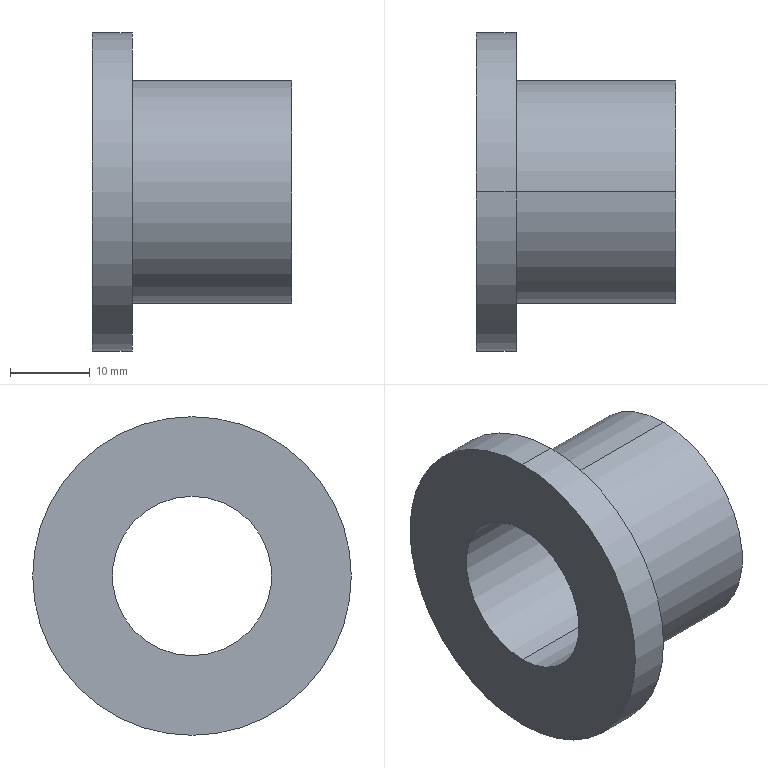Part | SolidWorks | features Revolution 1 | 1 solid | 9 faces | box 25 x 40 x 40 mm | volume 10744 mm3 | cylinder 6 | plane 3 | commonest cylinder face diameters 20 x2 28 x2 40 x2
STEP:
#1=CARTESIAN_POINT('',(25.,0.,24.));
#2=VERTEX_POINT('',#1);
#3=CARTESIAN_POINT('',(25.,0.,-4.));
#4=VERTEX_POINT('',#3);
#5=CARTESIAN_POINT('',(25.,0.,10.));
#6=DIRECTION('',(-1.,0.,0.));
#7=DIRECTION('',(0.,0.,1.));
#8=AXIS2_PLACEMENT_3D('',#5,#6,#7);
#9=CIRCLE('',#8,14.);
#10=EDGE_CURVE('',#2,#4,#9,.T.);
#11=ORIENTED_EDGE('',*,*,#10,.T.);
#12=CARTESIAN_POINT('',(5.,0.,-4.));
#13=VERTEX_POINT('',#12);
#14=CARTESIAN_POINT('',(0.,0.,-4.));
#15=DIRECTION('',(-1.,0.,0.));
#16=VECTOR('',#15,1000.);
#17=LINE('',#14,#16);
#18=EDGE_CURVE('',#4,#13,#17,.T.);
#19=ORIENTED_EDGE('',*,*,#18,.T.);
#20=CARTESIAN_POINT('',(5.,0.,24.));
#21=VERTEX_POINT('',#20);
#22=CARTESIAN_POINT('',(5.,0.,10.));
#23=DIRECTION('',(-1.,0.,0.));
#24=DIRECTION('',(0.,0.,1.));
#25=AXIS2_PLACEMENT_3D('',#22,#23,#24);
#26=CIRCLE('',#25,14.);
#27=EDGE_CURVE('',#21,#13,#26,.T.);
#28=ORIENTED_EDGE('',*,*,#27,.F.);
#29=CARTESIAN_POINT('',(0.,0.,24.));
#30=DIRECTION('',(-1.,0.,0.));
#31=VECTOR('',#30,1000.);
#32=LINE('',#29,#31);
#33=EDGE_CURVE('',#2,#21,#32,.T.);
#34=ORIENTED_EDGE('',*,*,#33,.F.);
#35=EDGE_LOOP('',(#11,#19,#28,#34));
#36=FACE_OUTER_BOUND('',#35,.T.);
#37=CARTESIAN_POINT('',(0.,0.,10.));
#38=DIRECTION('',(-1.,0.,0.));
#39=DIRECTION('',(0.,0.,1.));
#40=AXIS2_PLACEMENT_3D('',#37,#38,#39);
#41=CYLINDRICAL_SURFACE('',#40,14.);
#42=ADVANCED_FACE('',(#36),#41,.T.);
#43=CARTESIAN_POINT('',(5.,0.,30.));
#44=VERTEX_POINT('',#43);
#45=CARTESIAN_POINT('',(5.,0.,-10.));
#46=VERTEX_POINT('',#45);
#47=CARTESIAN_POINT('',(5.,0.,10.));
#48=DIRECTION('',(-1.,0.,0.));
#49=DIRECTION('',(0.,0.,1.));
#50=AXIS2_PLACEMENT_3D('',#47,#48,#49);
#51=CIRCLE('',#50,20.);
#52=EDGE_CURVE('',#44,#46,#51,.T.);
#53=ORIENTED_EDGE('',*,*,#52,.T.);
#54=CARTESIAN_POINT('',(0.,0.,-10.));
#55=VERTEX_POINT('',#54);
#56=CARTESIAN_POINT('',(0.,0.,-10.));
#57=DIRECTION('',(-1.,0.,0.));
#58=VECTOR('',#57,1000.);
#59=LINE('',#56,#58);
#60=EDGE_CURVE('',#46,#55,#59,.T.);
#61=ORIENTED_EDGE('',*,*,#60,.T.);
#62=CARTESIAN_POINT('',(0.,0.,30.));
#63=VERTEX_POINT('',#62);
#64=CARTESIAN_POINT('',(0.,0.,10.));
#65=DIRECTION('',(-1.,0.,0.));
#66=DIRECTION('',(0.,0.,1.));
#67=AXIS2_PLACEMENT_3D('',#64,#65,#66);
#68=CIRCLE('',#67,20.);
#69=EDGE_CURVE('',#63,#55,#68,.T.);
#70=ORIENTED_EDGE('',*,*,#69,.F.);
#71=CARTESIAN_POINT('',(0.,0.,30.));
#72=DIRECTION('',(-1.,0.,0.));
#73=VECTOR('',#72,1000.);
#74=LINE('',#71,#73);
#75=EDGE_CURVE('',#44,#63,#74,.T.);
#76=ORIENTED_EDGE('',*,*,#75,.F.);
#77=EDGE_LOOP('',(#53,#61,#70,#76));
#78=FACE_OUTER_BOUND('',#77,.T.);
#79=CARTESIAN_POINT('',(0.,0.,10.));
#80=DIRECTION('',(-1.,0.,0.));
#81=DIRECTION('',(0.,0.,1.));
#82=AXIS2_PLACEMENT_3D('',#79,#80,#81);
#83=CYLINDRICAL_SURFACE('',#82,20.);
#84=ADVANCED_FACE('',(#78),#83,.T.);
#85=CARTESIAN_POINT('',(25.,0.,0.));
#86=VERTEX_POINT('',#85);
#87=CARTESIAN_POINT('',(25.,0.,20.));
#88=VERTEX_POINT('',#87);
#89=CARTESIAN_POINT('',(25.,0.,10.));
#90=DIRECTION('',(-1.,0.,0.));
#91=DIRECTION('',(0.,0.,1.));
#92=AXIS2_PLACEMENT_3D('',#89,#90,#91);
#93=CIRCLE('',#92,10.);
#94=EDGE_CURVE('',#86,#88,#93,.T.);
#95=ORIENTED_EDGE('',*,*,#94,.F.);
#96=CARTESIAN_POINT('',(0.,0.,0.));
#97=VERTEX_POINT('',#96);
#98=CARTESIAN_POINT('',(0.,0.,0.));
#99=DIRECTION('',(-1.,0.,0.));
#100=VECTOR('',#99,1000.);
#101=LINE('',#98,#100);
#102=EDGE_CURVE('',#86,#97,#101,.T.);
#103=ORIENTED_EDGE('',*,*,#102,.T.);
#104=CARTESIAN_POINT('',(0.,0.,20.));
#105=VERTEX_POINT('',#104);
#106=CARTESIAN_POINT('',(0.,0.,10.));
#107=DIRECTION('',(-1.,0.,0.));
#108=DIRECTION('',(0.,0.,1.));
#109=AXIS2_PLACEMENT_3D('',#106,#107,#108);
#110=CIRCLE('',#109,10.);
#111=EDGE_CURVE('',#97,#105,#110,.T.);
#112=ORIENTED_EDGE('',*,*,#111,.T.);
#113=CARTESIAN_POINT('',(0.,0.,20.));
#114=DIRECTION('',(-1.,0.,0.));
#115=VECTOR('',#114,1000.);
#116=LINE('',#113,#115);
#117=EDGE_CURVE('',#88,#105,#116,.T.);
#118=ORIENTED_EDGE('',*,*,#117,.F.);
#119=EDGE_LOOP('',(#95,#103,#112,#118));
#120=FACE_OUTER_BOUND('',#119,.T.);
#121=CARTESIAN_POINT('',(0.,0.,10.));
#122=DIRECTION('',(-1.,0.,0.));
#123=DIRECTION('',(0.,0.,1.));
#124=AXIS2_PLACEMENT_3D('',#121,#122,#123);
#125=CYLINDRICAL_SURFACE('',#124,10.);
#126=ADVANCED_FACE('',(#120),#125,.F.);
#127=ORIENTED_EDGE('',*,*,#102,.F.);
#128=CARTESIAN_POINT('',(25.,0.,10.));
#129=DIRECTION('',(-1.,0.,0.));
#130=DIRECTION('',(0.,0.,1.));
#131=AXIS2_PLACEMENT_3D('',#128,#129,#130);
#132=CIRCLE('',#131,10.);
#133=EDGE_CURVE('',#88,#86,#132,.T.);
#134=ORIENTED_EDGE('',*,*,#133,.F.);
#135=ORIENTED_EDGE('',*,*,#117,.T.);
#136=CARTESIAN_POINT('',(0.,0.,10.));
#137=DIRECTION('',(-1.,0.,0.));
#138=DIRECTION('',(0.,0.,1.));
#139=AXIS2_PLACEMENT_3D('',#136,#137,#138);
#140=CIRCLE('',#139,10.);
#141=EDGE_CURVE('',#105,#97,#140,.T.);
#142=ORIENTED_EDGE('',*,*,#141,.T.);
#143=EDGE_LOOP('',(#127,#134,#135,#142));
#144=FACE_OUTER_BOUND('',#143,.T.);
#145=CARTESIAN_POINT('',(0.,0.,10.));
#146=DIRECTION('',(-1.,0.,0.));
#147=DIRECTION('',(0.,0.,1.));
#148=AXIS2_PLACEMENT_3D('',#145,#146,#147);
#149=CYLINDRICAL_SURFACE('',#148,10.);
#150=ADVANCED_FACE('',(#144),#149,.F.);
#151=ORIENTED_EDGE('',*,*,#141,.F.);
#152=ORIENTED_EDGE('',*,*,#111,.F.);
#153=EDGE_LOOP('',(#151,#152));
#154=FACE_BOUND('',#153,.T.);
#155=ORIENTED_EDGE('',*,*,#69,.T.);
#156=CARTESIAN_POINT('',(0.,0.,10.));
#157=DIRECTION('',(-1.,0.,0.));
#158=DIRECTION('',(0.,0.,1.));
#159=AXIS2_PLACEMENT_3D('',#156,#157,#158);
#160=CIRCLE('',#159,20.);
#161=EDGE_CURVE('',#55,#63,#160,.T.);
#162=ORIENTED_EDGE('',*,*,#161,.T.);
#163=EDGE_LOOP('',(#155,#162));
#164=FACE_OUTER_BOUND('',#163,.T.);
#165=CARTESIAN_POINT('',(0.,0.,0.));
#166=DIRECTION('',(1.,0.,0.));
#167=DIRECTION('',(0.,0.,-1.));
#168=AXIS2_PLACEMENT_3D('',#165,#166,#167);
#169=PLANE('',#168);
#170=ADVANCED_FACE('',(#154,#164),#169,.F.);
#171=ORIENTED_EDGE('',*,*,#60,.F.);
#172=CARTESIAN_POINT('',(5.,0.,10.));
#173=DIRECTION('',(-1.,0.,0.));
#174=DIRECTION('',(0.,0.,1.));
#175=AXIS2_PLACEMENT_3D('',#172,#173,#174);
#176=CIRCLE('',#175,20.);
#177=EDGE_CURVE('',#46,#44,#176,.T.);
#178=ORIENTED_EDGE('',*,*,#177,.T.);
#179=ORIENTED_EDGE('',*,*,#75,.T.);
#180=ORIENTED_EDGE('',*,*,#161,.F.);
#181=EDGE_LOOP('',(#171,#178,#179,#180));
#182=FACE_OUTER_BOUND('',#181,.T.);
#183=CARTESIAN_POINT('',(0.,0.,10.));
#184=DIRECTION('',(-1.,0.,0.));
#185=DIRECTION('',(0.,0.,1.));
#186=AXIS2_PLACEMENT_3D('',#183,#184,#185);
#187=CYLINDRICAL_SURFACE('',#186,20.);
#188=ADVANCED_FACE('',(#182),#187,.T.);
#189=ORIENTED_EDGE('',*,*,#52,.F.);
#190=ORIENTED_EDGE('',*,*,#177,.F.);
#191=EDGE_LOOP('',(#189,#190));
#192=FACE_OUTER_BOUND('',#191,.T.);
#193=ORIENTED_EDGE('',*,*,#27,.T.);
#194=CARTESIAN_POINT('',(5.,0.,10.));
#195=DIRECTION('',(-1.,0.,0.));
#196=DIRECTION('',(0.,0.,1.));
#197=AXIS2_PLACEMENT_3D('',#194,#195,#196);
#198=CIRCLE('',#197,14.);
#199=EDGE_CURVE('',#13,#21,#198,.T.);
#200=ORIENTED_EDGE('',*,*,#199,.T.);
#201=EDGE_LOOP('',(#193,#200));
#202=FACE_BOUND('',#201,.T.);
#203=CARTESIAN_POINT('',(5.,0.,-10.));
#204=DIRECTION('',(-1.,0.,0.));
#205=DIRECTION('',(0.,0.,1.));
#206=AXIS2_PLACEMENT_3D('',#203,#204,#205);
#207=PLANE('',#206);
#208=ADVANCED_FACE('',(#192,#202),#207,.F.);
#209=ORIENTED_EDGE('',*,*,#18,.F.);
#210=CARTESIAN_POINT('',(25.,0.,10.));
#211=DIRECTION('',(-1.,0.,0.));
#212=DIRECTION('',(0.,0.,1.));
#213=AXIS2_PLACEMENT_3D('',#210,#211,#212);
#214=CIRCLE('',#213,14.);
#215=EDGE_CURVE('',#4,#2,#214,.T.);
#216=ORIENTED_EDGE('',*,*,#215,.T.);
#217=ORIENTED_EDGE('',*,*,#33,.T.);
#218=ORIENTED_EDGE('',*,*,#199,.F.);
#219=EDGE_LOOP('',(#209,#216,#217,#218));
#220=FACE_OUTER_BOUND('',#219,.T.);
#221=CARTESIAN_POINT('',(0.,0.,10.));
#222=DIRECTION('',(-1.,0.,0.));
#223=DIRECTION('',(0.,0.,1.));
#224=AXIS2_PLACEMENT_3D('',#221,#222,#223);
#225=CYLINDRICAL_SURFACE('',#224,14.);
#226=ADVANCED_FACE('',(#220),#225,.T.);
#227=ORIENTED_EDGE('',*,*,#10,.F.);
#228=ORIENTED_EDGE('',*,*,#215,.F.);
#229=EDGE_LOOP('',(#227,#228));
#230=FACE_OUTER_BOUND('',#229,.T.);
#231=ORIENTED_EDGE('',*,*,#133,.T.);
#232=ORIENTED_EDGE('',*,*,#94,.T.);
#233=EDGE_LOOP('',(#231,#232));
#234=FACE_BOUND('',#233,.T.);
#235=CARTESIAN_POINT('',(25.,0.,-4.));
#236=DIRECTION('',(-1.,0.,0.));
#237=DIRECTION('',(0.,0.,1.));
#238=AXIS2_PLACEMENT_3D('',#235,#236,#237);
#239=PLANE('',#238);
#240=ADVANCED_FACE('',(#230,#234),#239,.F.);
#241=CLOSED_SHELL('',(#42,#84,#126,#150,#170,#188,#208,#226,#240));
#242=MANIFOLD_SOLID_BREP('',#241);
#243=CARTESIAN_POINT('',(0.,0.,0.));
#244=DIRECTION('',(0.,0.,1.));
#245=DIRECTION('',(1.,0.,0.));
#246=AXIS2_PLACEMENT_3D('',#243,#244,#245);
#247=(LENGTH_UNIT()NAMED_UNIT(*)SI_UNIT(.MILLI.,.METRE.));
#248=UNCERTAINTY_MEASURE_WITH_UNIT(LENGTH_MEASURE(0.00001),#247,'','');
#249=(NAMED_UNIT(*)PLANE_ANGLE_UNIT()SI_UNIT($,.RADIAN.));
#250=(NAMED_UNIT(*)SI_UNIT($,.STERADIAN.)SOLID_ANGLE_UNIT());
#251=(GEOMETRIC_REPRESENTATION_CONTEXT(3)GLOBAL_UNCERTAINTY_ASSIGNED_CONTEXT((#248))GLOBAL_UNIT_ASSIGNED_CONTEXT((#247,#249,#250))REPRESENTATION_CONTEXT('',''));
#252=ADVANCED_BREP_SHAPE_REPRESENTATION('',(#242,#246),#251);